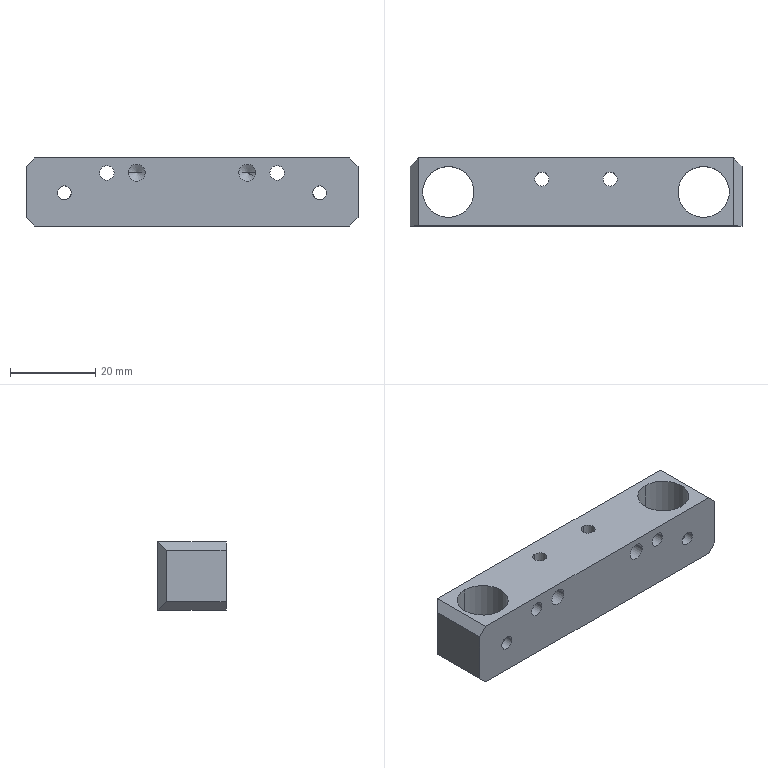NC program | NX | posted with a generic post | part box 78 x 16 x 16 mm
Lines 3609 to 3743 of 3743:
(PLANAR_MILL , TOOL : D6A45)
N7192 T01 M6
N7194 G54
N7196 G17 G0 G90 X-29.617 Y0.771 B0. C0. S7500 M3
N7198 G43 Z30. H1
N7200 Z1.
N7202 G94 G1 Z-1. F1250.
N7204 G3 X-30. Y0.95 R0.5
N7206 X-30.75 Y0.2 R0.75
N7208 X-30. Y0.95 R-0.75
N7210 X-30.383 Y0.771 R0.5
N7212 G1 Z1.
N7214 G0 Z30.
N7216 X-20.383 Y-5.121
N7218 Z1.
N7220 G1 Z-1.
N7222 G3 X-20. Y-5.3 R0.5
N7224 X-19.2 Y-4.5 R0.8
N7226 X-20. Y-5.3 R-0.8
N7228 X-19.617 Y-5.121 R0.5
N7230 G1 Z1.
N7232 G0 Z30.
N7234 X-13.766 Y-5.243
N7236 Z1.
N7238 G1 Z-1.
N7240 G3 X-13. Y-5.6 R1.
N7242 X-11.9 Y-4.5 R1.1
N7244 X-13. Y-5.6 R-1.1
N7246 X-12.234 Y-5.243 R1.
N7248 G1 Z1.
N7250 G0 Z30.
N7252 X0.766 Y-9.257
N7254 Z1.
N7256 G1 Z-1.
N7258 G3 X0. Y-8.9 R1.
N7260 G1 X-37.
N7262 G2 X-37.636 Y-8.636 R0.9
N7264 G1 X-39.636 Y-6.636
N7266 G2 X-39.9 Y-6. R0.9
N7268 G1 Y6.
N7270 G2 X-39.636 Y6.636 R0.9
N7272 G1 X-37.636 Y8.636
N7274 G2 X-37. Y8.9 R0.9
N7276 G1 X37.
N7278 G2 X37.636 Y8.636 R0.9
N7280 G1 X39.636 Y6.636
N7282 G2 X39.9 Y6. R0.9
N7284 G1 Y-6.
N7286 G2 X39.636 Y-6.636 R0.9
N7288 G1 X37.636 Y-8.636
N7290 G2 X37. Y-8.9 R0.9
N7292 G1 X0.
N7294 G3 X-0.766 Y-9.257 R1.
N7296 G1 Z1.
N7298 G0 Z30.
N7300 X12.234 Y-5.243
N7302 Z1.
N7304 G1 Z-1.
N7306 G3 X13. Y-5.6 R1.
N7308 X14.1 Y-4.5 R1.1
N7310 X13. Y-5.6 R-1.1
N7312 X13.766 Y-5.243 R1.
N7314 G1 Z1.
N7316 G0 Z30.
N7318 X19.617 Y-5.121
N7320 Z1.
N7322 G1 Z-1.
N7324 G3 X20. Y-5.3 R0.5
N7326 X20.8 Y-4.5 R0.8
N7328 X20. Y-5.3 R-0.8
N7330 X20.383 Y-5.121 R0.5
N7332 G1 Z1.
N7334 G0 Z30.
N7336 X30.383 Y0.771
N7338 Z1.
N7340 G1 Z-1.
N7342 G3 X30. Y0.95 R0.5
N7344 X29.25 Y0.2 R0.75
N7346 X30. Y0.95 R-0.75
N7348 X29.617 Y0.771 R0.5
N7350 G1 Z1.
N7352 G0 Z30.
N7354 M5
(刀补18 , TOOL : D2)
N7356 T18 M6
N7358 G54
N7360 G17 G0 G90 X-13. Y-4.5 B0. C0. S7500 M3
N7362 G43 Z30. H18
N7364 Z0.5
N7366 G41 G94 G1 X-13.003 Y-4.4 F800. D18
N7368 G3 X-13.98 Y-4.5 R0.494
N7370 X-13.98 Y-4.5 Z-0.5 I0.98 J0.
N7372 X-13.98 Y-4.5 Z-1.5 I0.98 J0.
N7374 X-13.98 Y-4.5 Z-2.5 I0.98 J0.
N7376 X-13.98 Y-4.5 Z-3.5 I0.98 J0.
N7378 X-13.98 Y-4.5 Z-4.5 I0.98 J0.
N7380 X-13.98 Y-4.5 Z-5.5 I0.98 J0.
N7382 X-13.98 Y-4.5 Z-6.5 I0.98 J0.
N7384 X-13.98 Y-4.5 Z-7.5 I0.98 J0.
N7386 X-13.98 Y-4.5 Z-8.5 I0.98 J0.
N7388 X-13.98 Y-4.5 Z-9.5 I0.98 J0.
N7390 X-12.02 Y-4.5 Z-10. I0.98 J0.
N7392 X-13. Y-3.52 R0.98
N7394 X-12.02 Y-4.5 R-0.98
N7396 X-12.997 Y-4.4 R0.494
N7398 G40
N7400 G1 X-13. Y-4.5
N7402 G0 Z30.
N7404 X13.
N7406 Z0.5
N7408 G41 G1 X12.997 Y-4.4
N7410 G3 X12.02 Y-4.5 R0.494
N7412 X12.02 Y-4.5 Z-0.5 I0.98 J0.
N7414 X12.02 Y-4.5 Z-1.5 I0.98 J0.
N7416 X12.02 Y-4.5 Z-2.5 I0.98 J0.
N7418 X12.02 Y-4.5 Z-3.5 I0.98 J0.
N7420 X12.02 Y-4.5 Z-4.5 I0.98 J0.
N7422 X12.02 Y-4.5 Z-5.5 I0.98 J0.
N7424 X12.02 Y-4.5 Z-6.5 I0.98 J0.
N7426 X12.02 Y-4.5 Z-7.5 I0.98 J0.
N7428 X12.02 Y-4.5 Z-8.5 I0.98 J0.
N7430 X12.02 Y-4.5 Z-9.5 I0.98 J0.
N7432 X13.98 Y-4.5 Z-10. I0.98 J0.
N7434 X13. Y-3.52 R0.98
N7436 X13.98 Y-4.5 R-0.98
N7438 X13.003 Y-4.4 R0.494
N7440 G40
N7442 G1 X13. Y-4.5
N7444 G0 Z30.
N7446 M5
N7448 M2